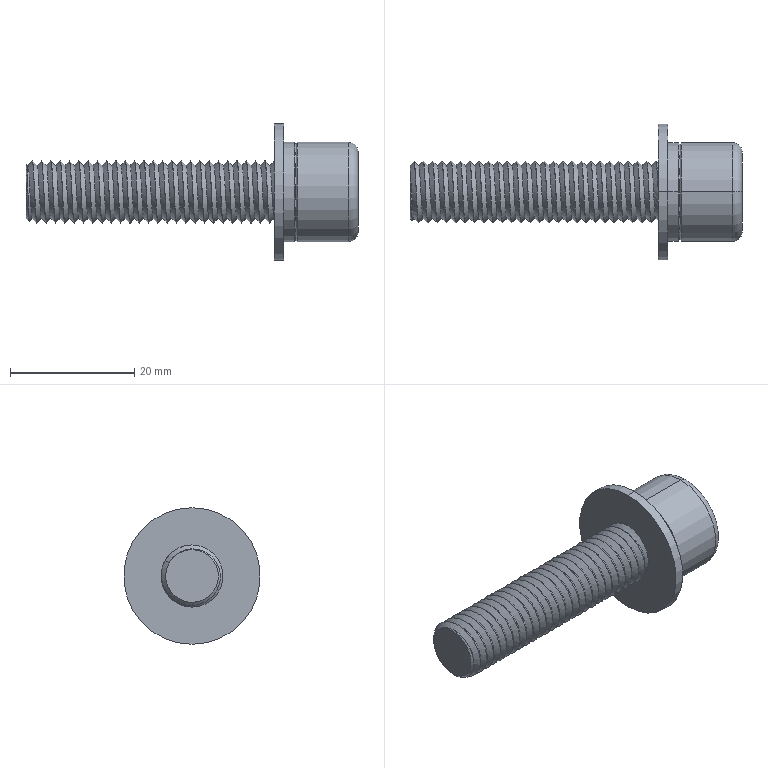Part | SolidWorks | features BaseBody 1 | 1 solid | 81 faces | box 53.5 x 22 x 22 mm | volume 5383 mm3 | cylinder 59 | plane 11 | cone 7 | spline 2 | torus 2 | commonest cylinder face diameters 10 x53 16 x4 22 x2